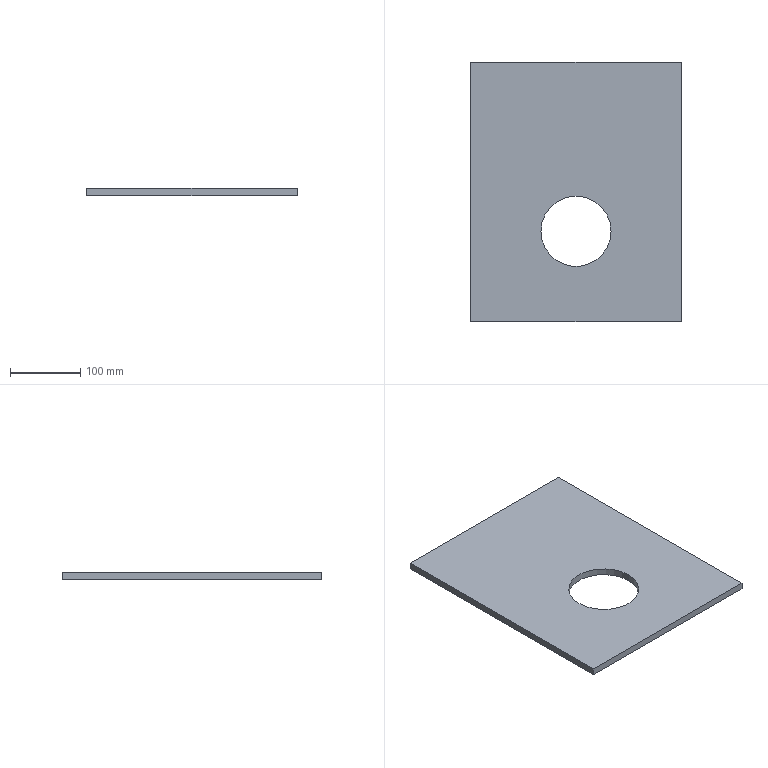Part | SolidWorks | features Extrusion 1 | 1 solid | 8 faces | box 300 x 370 x 10 mm | volume 1031460 mm3 | plane 6 | cylinder 2 | commonest cylinder face diameters 100 x2
STEP:
#1=CARTESIAN_POINT('',(100.,129.,10.));
#2=VERTEX_POINT('',#1);
#3=CARTESIAN_POINT('',(200.,129.,10.));
#4=VERTEX_POINT('',#3);
#5=CARTESIAN_POINT('',(150.,129.,10.));
#6=DIRECTION('',(0.,0.,1.));
#7=DIRECTION('',(1.,0.,0.));
#8=AXIS2_PLACEMENT_3D('',#5,#6,#7);
#9=CIRCLE('',#8,50.);
#10=EDGE_CURVE('',#2,#4,#9,.T.);
#11=ORIENTED_EDGE('',*,*,#10,.T.);
#12=CARTESIAN_POINT('',(200.,129.,0.));
#13=VERTEX_POINT('',#12);
#14=CARTESIAN_POINT('',(200.,129.,10.));
#15=DIRECTION('',(0.,0.,-1.));
#16=VECTOR('',#15,1000.);
#17=LINE('',#14,#16);
#18=EDGE_CURVE('',#4,#13,#17,.T.);
#19=ORIENTED_EDGE('',*,*,#18,.T.);
#20=CARTESIAN_POINT('',(100.,129.,0.));
#21=VERTEX_POINT('',#20);
#22=CARTESIAN_POINT('',(150.,129.,0.));
#23=DIRECTION('',(0.,0.,1.));
#24=DIRECTION('',(1.,0.,0.));
#25=AXIS2_PLACEMENT_3D('',#22,#23,#24);
#26=CIRCLE('',#25,50.);
#27=EDGE_CURVE('',#21,#13,#26,.T.);
#28=ORIENTED_EDGE('',*,*,#27,.F.);
#29=CARTESIAN_POINT('',(100.,129.,10.));
#30=DIRECTION('',(0.,0.,-1.));
#31=VECTOR('',#30,1000.);
#32=LINE('',#29,#31);
#33=EDGE_CURVE('',#2,#21,#32,.T.);
#34=ORIENTED_EDGE('',*,*,#33,.F.);
#35=EDGE_LOOP('',(#11,#19,#28,#34));
#36=FACE_OUTER_BOUND('',#35,.T.);
#37=CARTESIAN_POINT('',(150.,129.,10.));
#38=DIRECTION('',(0.,0.,-1.));
#39=DIRECTION('',(-1.,0.,0.));
#40=AXIS2_PLACEMENT_3D('',#37,#38,#39);
#41=CYLINDRICAL_SURFACE('',#40,50.);
#42=ADVANCED_FACE('',(#36),#41,.F.);
#43=CARTESIAN_POINT('',(0.,370.,10.));
#44=VERTEX_POINT('',#43);
#45=CARTESIAN_POINT('',(0.,0.,10.));
#46=VERTEX_POINT('',#45);
#47=CARTESIAN_POINT('',(0.,0.,10.));
#48=DIRECTION('',(0.,-1.,0.));
#49=VECTOR('',#48,1000.);
#50=LINE('',#47,#49);
#51=EDGE_CURVE('',#44,#46,#50,.T.);
#52=ORIENTED_EDGE('',*,*,#51,.T.);
#53=CARTESIAN_POINT('',(300.,0.,10.));
#54=VERTEX_POINT('',#53);
#55=CARTESIAN_POINT('',(0.,0.,10.));
#56=DIRECTION('',(1.,0.,0.));
#57=VECTOR('',#56,1000.);
#58=LINE('',#55,#57);
#59=EDGE_CURVE('',#46,#54,#58,.T.);
#60=ORIENTED_EDGE('',*,*,#59,.T.);
#61=CARTESIAN_POINT('',(300.,370.,10.));
#62=VERTEX_POINT('',#61);
#63=CARTESIAN_POINT('',(300.,0.,10.));
#64=DIRECTION('',(0.,1.,0.));
#65=VECTOR('',#64,1000.);
#66=LINE('',#63,#65);
#67=EDGE_CURVE('',#54,#62,#66,.T.);
#68=ORIENTED_EDGE('',*,*,#67,.T.);
#69=CARTESIAN_POINT('',(0.,370.,10.));
#70=DIRECTION('',(-1.,0.,0.));
#71=VECTOR('',#70,1000.);
#72=LINE('',#69,#71);
#73=EDGE_CURVE('',#62,#44,#72,.T.);
#74=ORIENTED_EDGE('',*,*,#73,.T.);
#75=EDGE_LOOP('',(#52,#60,#68,#74));
#76=FACE_OUTER_BOUND('',#75,.T.);
#77=ORIENTED_EDGE('',*,*,#10,.F.);
#78=CARTESIAN_POINT('',(150.,129.,10.));
#79=DIRECTION('',(0.,0.,1.));
#80=DIRECTION('',(1.,0.,0.));
#81=AXIS2_PLACEMENT_3D('',#78,#79,#80);
#82=CIRCLE('',#81,50.);
#83=EDGE_CURVE('',#4,#2,#82,.T.);
#84=ORIENTED_EDGE('',*,*,#83,.F.);
#85=EDGE_LOOP('',(#77,#84));
#86=FACE_BOUND('',#85,.T.);
#87=CARTESIAN_POINT('',(0.,370.,10.));
#88=DIRECTION('',(0.,0.,-1.));
#89=DIRECTION('',(-1.,0.,0.));
#90=AXIS2_PLACEMENT_3D('',#87,#88,#89);
#91=PLANE('',#90);
#92=ADVANCED_FACE('',(#76,#86),#91,.F.);
#93=CARTESIAN_POINT('',(0.,370.,0.));
#94=VERTEX_POINT('',#93);
#95=CARTESIAN_POINT('',(0.,0.,0.));
#96=VERTEX_POINT('',#95);
#97=CARTESIAN_POINT('',(0.,0.,0.));
#98=DIRECTION('',(0.,-1.,0.));
#99=VECTOR('',#98,1000.);
#100=LINE('',#97,#99);
#101=EDGE_CURVE('',#94,#96,#100,.T.);
#102=ORIENTED_EDGE('',*,*,#101,.F.);
#103=CARTESIAN_POINT('',(300.,370.,0.));
#104=VERTEX_POINT('',#103);
#105=CARTESIAN_POINT('',(0.,370.,0.));
#106=DIRECTION('',(-1.,0.,0.));
#107=VECTOR('',#106,1000.);
#108=LINE('',#105,#107);
#109=EDGE_CURVE('',#104,#94,#108,.T.);
#110=ORIENTED_EDGE('',*,*,#109,.F.);
#111=CARTESIAN_POINT('',(300.,0.,0.));
#112=VERTEX_POINT('',#111);
#113=CARTESIAN_POINT('',(300.,0.,0.));
#114=DIRECTION('',(0.,1.,0.));
#115=VECTOR('',#114,1000.);
#116=LINE('',#113,#115);
#117=EDGE_CURVE('',#112,#104,#116,.T.);
#118=ORIENTED_EDGE('',*,*,#117,.F.);
#119=CARTESIAN_POINT('',(0.,0.,0.));
#120=DIRECTION('',(1.,0.,0.));
#121=VECTOR('',#120,1000.);
#122=LINE('',#119,#121);
#123=EDGE_CURVE('',#96,#112,#122,.T.);
#124=ORIENTED_EDGE('',*,*,#123,.F.);
#125=EDGE_LOOP('',(#102,#110,#118,#124));
#126=FACE_OUTER_BOUND('',#125,.T.);
#127=ORIENTED_EDGE('',*,*,#27,.T.);
#128=CARTESIAN_POINT('',(150.,129.,0.));
#129=DIRECTION('',(0.,0.,1.));
#130=DIRECTION('',(1.,0.,0.));
#131=AXIS2_PLACEMENT_3D('',#128,#129,#130);
#132=CIRCLE('',#131,50.);
#133=EDGE_CURVE('',#13,#21,#132,.T.);
#134=ORIENTED_EDGE('',*,*,#133,.T.);
#135=EDGE_LOOP('',(#127,#134));
#136=FACE_BOUND('',#135,.T.);
#137=CARTESIAN_POINT('',(0.,370.,0.));
#138=DIRECTION('',(0.,0.,-1.));
#139=DIRECTION('',(-1.,0.,0.));
#140=AXIS2_PLACEMENT_3D('',#137,#138,#139);
#141=PLANE('',#140);
#142=ADVANCED_FACE('',(#126,#136),#141,.T.);
#143=ORIENTED_EDGE('',*,*,#101,.T.);
#144=CARTESIAN_POINT('',(0.,0.,10.));
#145=DIRECTION('',(0.,0.,-1.));
#146=VECTOR('',#145,1000.);
#147=LINE('',#144,#146);
#148=EDGE_CURVE('',#46,#96,#147,.T.);
#149=ORIENTED_EDGE('',*,*,#148,.F.);
#150=ORIENTED_EDGE('',*,*,#51,.F.);
#151=CARTESIAN_POINT('',(0.,370.,10.));
#152=DIRECTION('',(0.,0.,-1.));
#153=VECTOR('',#152,1000.);
#154=LINE('',#151,#153);
#155=EDGE_CURVE('',#44,#94,#154,.T.);
#156=ORIENTED_EDGE('',*,*,#155,.T.);
#157=EDGE_LOOP('',(#143,#149,#150,#156));
#158=FACE_OUTER_BOUND('',#157,.T.);
#159=CARTESIAN_POINT('',(0.,0.,10.));
#160=DIRECTION('',(1.,0.,0.));
#161=DIRECTION('',(0.,0.,-1.));
#162=AXIS2_PLACEMENT_3D('',#159,#160,#161);
#163=PLANE('',#162);
#164=ADVANCED_FACE('',(#158),#163,.F.);
#165=ORIENTED_EDGE('',*,*,#123,.T.);
#166=CARTESIAN_POINT('',(300.,0.,10.));
#167=DIRECTION('',(0.,0.,-1.));
#168=VECTOR('',#167,1000.);
#169=LINE('',#166,#168);
#170=EDGE_CURVE('',#54,#112,#169,.T.);
#171=ORIENTED_EDGE('',*,*,#170,.F.);
#172=ORIENTED_EDGE('',*,*,#59,.F.);
#173=ORIENTED_EDGE('',*,*,#148,.T.);
#174=EDGE_LOOP('',(#165,#171,#172,#173));
#175=FACE_OUTER_BOUND('',#174,.T.);
#176=CARTESIAN_POINT('',(0.,0.,10.));
#177=DIRECTION('',(0.,1.,0.));
#178=DIRECTION('',(0.,0.,1.));
#179=AXIS2_PLACEMENT_3D('',#176,#177,#178);
#180=PLANE('',#179);
#181=ADVANCED_FACE('',(#175),#180,.F.);
#182=ORIENTED_EDGE('',*,*,#117,.T.);
#183=CARTESIAN_POINT('',(300.,370.,10.));
#184=DIRECTION('',(0.,0.,-1.));
#185=VECTOR('',#184,1000.);
#186=LINE('',#183,#185);
#187=EDGE_CURVE('',#62,#104,#186,.T.);
#188=ORIENTED_EDGE('',*,*,#187,.F.);
#189=ORIENTED_EDGE('',*,*,#67,.F.);
#190=ORIENTED_EDGE('',*,*,#170,.T.);
#191=EDGE_LOOP('',(#182,#188,#189,#190));
#192=FACE_OUTER_BOUND('',#191,.T.);
#193=CARTESIAN_POINT('',(300.,0.,10.));
#194=DIRECTION('',(-1.,0.,0.));
#195=DIRECTION('',(0.,0.,1.));
#196=AXIS2_PLACEMENT_3D('',#193,#194,#195);
#197=PLANE('',#196);
#198=ADVANCED_FACE('',(#192),#197,.F.);
#199=ORIENTED_EDGE('',*,*,#109,.T.);
#200=ORIENTED_EDGE('',*,*,#155,.F.);
#201=ORIENTED_EDGE('',*,*,#73,.F.);
#202=ORIENTED_EDGE('',*,*,#187,.T.);
#203=EDGE_LOOP('',(#199,#200,#201,#202));
#204=FACE_OUTER_BOUND('',#203,.T.);
#205=CARTESIAN_POINT('',(0.,370.,10.));
#206=DIRECTION('',(0.,-1.,0.));
#207=DIRECTION('',(0.,0.,-1.));
#208=AXIS2_PLACEMENT_3D('',#205,#206,#207);
#209=PLANE('',#208);
#210=ADVANCED_FACE('',(#204),#209,.F.);
#211=ORIENTED_EDGE('',*,*,#18,.F.);
#212=ORIENTED_EDGE('',*,*,#83,.T.);
#213=ORIENTED_EDGE('',*,*,#33,.T.);
#214=ORIENTED_EDGE('',*,*,#133,.F.);
#215=EDGE_LOOP('',(#211,#212,#213,#214));
#216=FACE_OUTER_BOUND('',#215,.T.);
#217=CARTESIAN_POINT('',(150.,129.,10.));
#218=DIRECTION('',(0.,0.,-1.));
#219=DIRECTION('',(-1.,0.,0.));
#220=AXIS2_PLACEMENT_3D('',#217,#218,#219);
#221=CYLINDRICAL_SURFACE('',#220,50.);
#222=ADVANCED_FACE('',(#216),#221,.F.);
#223=CLOSED_SHELL('',(#42,#92,#142,#164,#181,#198,#210,#222));
#224=MANIFOLD_SOLID_BREP('',#223);
#225=CARTESIAN_POINT('',(0.,0.,0.));
#226=DIRECTION('',(0.,0.,1.));
#227=DIRECTION('',(1.,0.,0.));
#228=AXIS2_PLACEMENT_3D('',#225,#226,#227);
#229=(LENGTH_UNIT()NAMED_UNIT(*)SI_UNIT(.MILLI.,.METRE.));
#230=UNCERTAINTY_MEASURE_WITH_UNIT(LENGTH_MEASURE(0.00001),#229,'','');
#231=(NAMED_UNIT(*)PLANE_ANGLE_UNIT()SI_UNIT($,.RADIAN.));
#232=(NAMED_UNIT(*)SI_UNIT($,.STERADIAN.)SOLID_ANGLE_UNIT());
#233=(GEOMETRIC_REPRESENTATION_CONTEXT(3)GLOBAL_UNCERTAINTY_ASSIGNED_CONTEXT((#230))GLOBAL_UNIT_ASSIGNED_CONTEXT((#229,#231,#232))REPRESENTATION_CONTEXT('',''));
#234=ADVANCED_BREP_SHAPE_REPRESENTATION('',(#224,#228),#233);